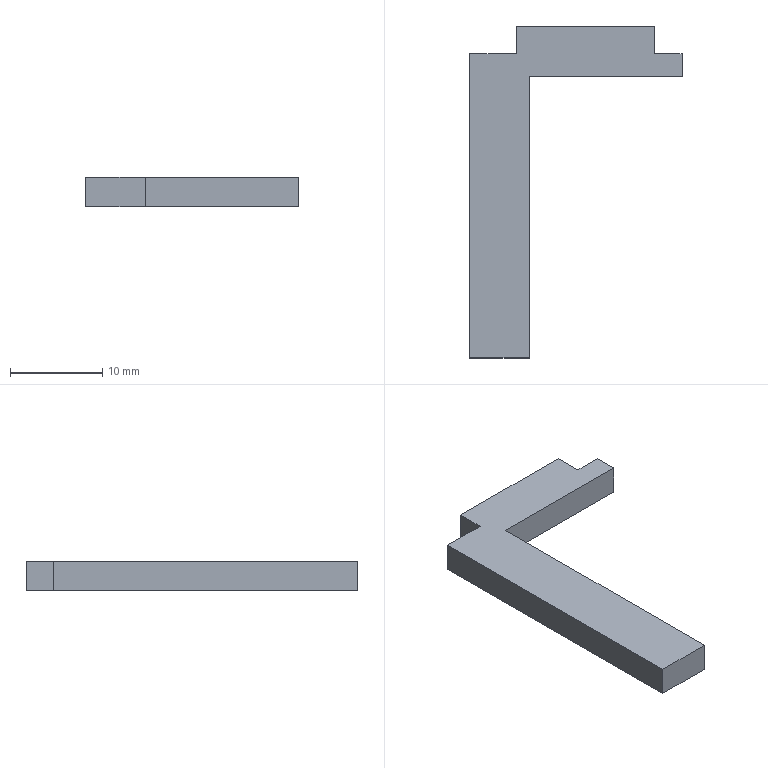Part | SolidWorks | features FlatPattern 1, SMBaseFlange 1, SheetMetal 1 | 1 solid | 12 faces | box 23 x 36 x 3.2 mm | volume 953.226 mm3 | plane 12
STEP:
#1=CARTESIAN_POINT('',(2.154,0.,0.));
#2=VERTEX_POINT('',#1);
#3=CARTESIAN_POINT('',(-0.8457,0.,0.));
#4=VERTEX_POINT('',#3);
#5=CARTESIAN_POINT('',(2.154,0.,0.));
#6=DIRECTION('',(-1.,0.,0.));
#7=VECTOR('',#6,1000.);
#8=LINE('',#5,#7);
#9=EDGE_CURVE('',#2,#4,#8,.T.);
#10=ORIENTED_EDGE('',*,*,#9,.T.);
#11=CARTESIAN_POINT('',(-0.8457,0.,3.2));
#12=VERTEX_POINT('',#11);
#13=CARTESIAN_POINT('',(-0.8457,0.,3.2));
#14=DIRECTION('',(0.,0.,-1.));
#15=VECTOR('',#14,1000.);
#16=LINE('',#13,#15);
#17=EDGE_CURVE('',#12,#4,#16,.T.);
#18=ORIENTED_EDGE('',*,*,#17,.F.);
#19=CARTESIAN_POINT('',(2.154,0.,3.2));
#20=VERTEX_POINT('',#19);
#21=CARTESIAN_POINT('',(2.154,0.,3.2));
#22=DIRECTION('',(-1.,0.,0.));
#23=VECTOR('',#22,1000.);
#24=LINE('',#21,#23);
#25=EDGE_CURVE('',#20,#12,#24,.T.);
#26=ORIENTED_EDGE('',*,*,#25,.F.);
#27=CARTESIAN_POINT('',(2.154,0.,3.2));
#28=DIRECTION('',(0.,0.,-1.));
#29=VECTOR('',#28,1000.);
#30=LINE('',#27,#29);
#31=EDGE_CURVE('',#20,#2,#30,.T.);
#32=ORIENTED_EDGE('',*,*,#31,.T.);
#33=EDGE_LOOP('',(#10,#18,#26,#32));
#34=FACE_OUTER_BOUND('',#33,.T.);
#35=CARTESIAN_POINT('',(2.154,0.,3.2));
#36=DIRECTION('',(0.,-1.,0.));
#37=DIRECTION('',(0.,0.,-1.));
#38=AXIS2_PLACEMENT_3D('',#35,#36,#37);
#39=PLANE('',#38);
#40=ADVANCED_FACE('',(#34),#39,.F.);
#41=CARTESIAN_POINT('',(-0.8457,3.,0.));
#42=VERTEX_POINT('',#41);
#43=CARTESIAN_POINT('',(-0.8457,0.,0.));
#44=DIRECTION('',(0.,1.,0.));
#45=VECTOR('',#44,1000.);
#46=LINE('',#43,#45);
#47=EDGE_CURVE('',#4,#42,#46,.T.);
#48=ORIENTED_EDGE('',*,*,#47,.T.);
#49=CARTESIAN_POINT('',(-0.8457,3.,3.2));
#50=VERTEX_POINT('',#49);
#51=CARTESIAN_POINT('',(-0.8457,3.,3.2));
#52=DIRECTION('',(0.,0.,-1.));
#53=VECTOR('',#52,1000.);
#54=LINE('',#51,#53);
#55=EDGE_CURVE('',#50,#42,#54,.T.);
#56=ORIENTED_EDGE('',*,*,#55,.F.);
#57=CARTESIAN_POINT('',(-0.8457,0.,3.2));
#58=DIRECTION('',(0.,1.,0.));
#59=VECTOR('',#58,1000.);
#60=LINE('',#57,#59);
#61=EDGE_CURVE('',#12,#50,#60,.T.);
#62=ORIENTED_EDGE('',*,*,#61,.F.);
#63=ORIENTED_EDGE('',*,*,#17,.T.);
#64=EDGE_LOOP('',(#48,#56,#62,#63));
#65=FACE_OUTER_BOUND('',#64,.T.);
#66=CARTESIAN_POINT('',(-0.8457,0.,3.2));
#67=DIRECTION('',(-1.,0.,0.));
#68=DIRECTION('',(0.,-1.,0.));
#69=AXIS2_PLACEMENT_3D('',#66,#67,#68);
#70=PLANE('',#69);
#71=ADVANCED_FACE('',(#65),#70,.F.);
#72=CARTESIAN_POINT('',(-15.846,3.,0.));
#73=VERTEX_POINT('',#72);
#74=CARTESIAN_POINT('',(-0.8457,3.,0.));
#75=DIRECTION('',(-1.,0.,0.));
#76=VECTOR('',#75,1000.);
#77=LINE('',#74,#76);
#78=EDGE_CURVE('',#42,#73,#77,.T.);
#79=ORIENTED_EDGE('',*,*,#78,.T.);
#80=CARTESIAN_POINT('',(-15.846,3.,3.2));
#81=VERTEX_POINT('',#80);
#82=CARTESIAN_POINT('',(-15.846,3.,3.2));
#83=DIRECTION('',(0.,0.,-1.));
#84=VECTOR('',#83,1000.);
#85=LINE('',#82,#84);
#86=EDGE_CURVE('',#81,#73,#85,.T.);
#87=ORIENTED_EDGE('',*,*,#86,.F.);
#88=CARTESIAN_POINT('',(-0.8457,3.,3.2));
#89=DIRECTION('',(-1.,0.,0.));
#90=VECTOR('',#89,1000.);
#91=LINE('',#88,#90);
#92=EDGE_CURVE('',#50,#81,#91,.T.);
#93=ORIENTED_EDGE('',*,*,#92,.F.);
#94=ORIENTED_EDGE('',*,*,#55,.T.);
#95=EDGE_LOOP('',(#79,#87,#93,#94));
#96=FACE_OUTER_BOUND('',#95,.T.);
#97=CARTESIAN_POINT('',(-0.8457,3.,3.2));
#98=DIRECTION('',(0.,-1.,0.));
#99=DIRECTION('',(1.,0.,0.));
#100=AXIS2_PLACEMENT_3D('',#97,#98,#99);
#101=PLANE('',#100);
#102=ADVANCED_FACE('',(#96),#101,.F.);
#103=CARTESIAN_POINT('',(-15.846,0.,0.));
#104=VERTEX_POINT('',#103);
#105=CARTESIAN_POINT('',(-15.846,3.,0.));
#106=DIRECTION('',(0.,-1.,0.));
#107=VECTOR('',#106,1000.);
#108=LINE('',#105,#107);
#109=EDGE_CURVE('',#73,#104,#108,.T.);
#110=ORIENTED_EDGE('',*,*,#109,.T.);
#111=CARTESIAN_POINT('',(-15.846,0.,3.2));
#112=VERTEX_POINT('',#111);
#113=CARTESIAN_POINT('',(-15.846,0.,3.2));
#114=DIRECTION('',(0.,0.,-1.));
#115=VECTOR('',#114,1000.);
#116=LINE('',#113,#115);
#117=EDGE_CURVE('',#112,#104,#116,.T.);
#118=ORIENTED_EDGE('',*,*,#117,.F.);
#119=CARTESIAN_POINT('',(-15.846,3.,3.2));
#120=DIRECTION('',(0.,-1.,0.));
#121=VECTOR('',#120,1000.);
#122=LINE('',#119,#121);
#123=EDGE_CURVE('',#81,#112,#122,.T.);
#124=ORIENTED_EDGE('',*,*,#123,.F.);
#125=ORIENTED_EDGE('',*,*,#86,.T.);
#126=EDGE_LOOP('',(#110,#118,#124,#125));
#127=FACE_OUTER_BOUND('',#126,.T.);
#128=CARTESIAN_POINT('',(-15.846,3.,3.2));
#129=DIRECTION('',(1.,0.,0.));
#130=DIRECTION('',(0.,0.,-1.));
#131=AXIS2_PLACEMENT_3D('',#128,#129,#130);
#132=PLANE('',#131);
#133=ADVANCED_FACE('',(#127),#132,.F.);
#134=CARTESIAN_POINT('',(-20.846,0.,0.));
#135=VERTEX_POINT('',#134);
#136=CARTESIAN_POINT('',(-15.846,0.,0.));
#137=DIRECTION('',(-1.,0.,0.));
#138=VECTOR('',#137,1000.);
#139=LINE('',#136,#138);
#140=EDGE_CURVE('',#104,#135,#139,.T.);
#141=ORIENTED_EDGE('',*,*,#140,.T.);
#142=CARTESIAN_POINT('',(-20.846,0.,3.2));
#143=VERTEX_POINT('',#142);
#144=CARTESIAN_POINT('',(-20.846,0.,3.2));
#145=DIRECTION('',(0.,0.,-1.));
#146=VECTOR('',#145,1000.);
#147=LINE('',#144,#146);
#148=EDGE_CURVE('',#143,#135,#147,.T.);
#149=ORIENTED_EDGE('',*,*,#148,.F.);
#150=CARTESIAN_POINT('',(-15.846,0.,3.2));
#151=DIRECTION('',(-1.,0.,0.));
#152=VECTOR('',#151,1000.);
#153=LINE('',#150,#152);
#154=EDGE_CURVE('',#112,#143,#153,.T.);
#155=ORIENTED_EDGE('',*,*,#154,.F.);
#156=ORIENTED_EDGE('',*,*,#117,.T.);
#157=EDGE_LOOP('',(#141,#149,#155,#156));
#158=FACE_OUTER_BOUND('',#157,.T.);
#159=CARTESIAN_POINT('',(-15.846,0.,3.2));
#160=DIRECTION('',(0.,-1.,0.));
#161=DIRECTION('',(1.,0.,0.));
#162=AXIS2_PLACEMENT_3D('',#159,#160,#161);
#163=PLANE('',#162);
#164=ADVANCED_FACE('',(#158),#163,.F.);
#165=CARTESIAN_POINT('',(-20.846,-33.,0.));
#166=VERTEX_POINT('',#165);
#167=CARTESIAN_POINT('',(-20.846,0.,0.));
#168=DIRECTION('',(0.,-1.,0.));
#169=VECTOR('',#168,1000.);
#170=LINE('',#167,#169);
#171=EDGE_CURVE('',#135,#166,#170,.T.);
#172=ORIENTED_EDGE('',*,*,#171,.T.);
#173=CARTESIAN_POINT('',(-20.846,-33.,3.2));
#174=VERTEX_POINT('',#173);
#175=CARTESIAN_POINT('',(-20.846,-33.,3.2));
#176=DIRECTION('',(0.,0.,-1.));
#177=VECTOR('',#176,1000.);
#178=LINE('',#175,#177);
#179=EDGE_CURVE('',#174,#166,#178,.T.);
#180=ORIENTED_EDGE('',*,*,#179,.F.);
#181=CARTESIAN_POINT('',(-20.846,0.,3.2));
#182=DIRECTION('',(0.,-1.,0.));
#183=VECTOR('',#182,1000.);
#184=LINE('',#181,#183);
#185=EDGE_CURVE('',#143,#174,#184,.T.);
#186=ORIENTED_EDGE('',*,*,#185,.F.);
#187=ORIENTED_EDGE('',*,*,#148,.T.);
#188=EDGE_LOOP('',(#172,#180,#186,#187));
#189=FACE_OUTER_BOUND('',#188,.T.);
#190=CARTESIAN_POINT('',(-20.846,0.,3.2));
#191=DIRECTION('',(1.,0.,0.));
#192=DIRECTION('',(0.,1.,0.));
#193=AXIS2_PLACEMENT_3D('',#190,#191,#192);
#194=PLANE('',#193);
#195=ADVANCED_FACE('',(#189),#194,.F.);
#196=CARTESIAN_POINT('',(-14.44,-33.,0.));
#197=VERTEX_POINT('',#196);
#198=CARTESIAN_POINT('',(-20.846,-33.,0.));
#199=DIRECTION('',(1.,0.,0.));
#200=VECTOR('',#199,1000.);
#201=LINE('',#198,#200);
#202=EDGE_CURVE('',#166,#197,#201,.T.);
#203=ORIENTED_EDGE('',*,*,#202,.T.);
#204=CARTESIAN_POINT('',(-14.44,-33.,3.2));
#205=VERTEX_POINT('',#204);
#206=CARTESIAN_POINT('',(-14.44,-33.,3.2));
#207=DIRECTION('',(0.,0.,-1.));
#208=VECTOR('',#207,1000.);
#209=LINE('',#206,#208);
#210=EDGE_CURVE('',#205,#197,#209,.T.);
#211=ORIENTED_EDGE('',*,*,#210,.F.);
#212=CARTESIAN_POINT('',(-20.846,-33.,3.2));
#213=DIRECTION('',(1.,0.,0.));
#214=VECTOR('',#213,1000.);
#215=LINE('',#212,#214);
#216=EDGE_CURVE('',#174,#205,#215,.T.);
#217=ORIENTED_EDGE('',*,*,#216,.F.);
#218=ORIENTED_EDGE('',*,*,#179,.T.);
#219=EDGE_LOOP('',(#203,#211,#217,#218));
#220=FACE_OUTER_BOUND('',#219,.T.);
#221=CARTESIAN_POINT('',(-20.846,-33.,3.2));
#222=DIRECTION('',(0.,1.,0.));
#223=DIRECTION('',(0.,0.,1.));
#224=AXIS2_PLACEMENT_3D('',#221,#222,#223);
#225=PLANE('',#224);
#226=ADVANCED_FACE('',(#220),#225,.F.);
#227=CARTESIAN_POINT('',(-14.44,-2.5,0.));
#228=VERTEX_POINT('',#227);
#229=CARTESIAN_POINT('',(-14.44,-33.,0.));
#230=DIRECTION('',(0.,1.,0.));
#231=VECTOR('',#230,1000.);
#232=LINE('',#229,#231);
#233=EDGE_CURVE('',#197,#228,#232,.T.);
#234=ORIENTED_EDGE('',*,*,#233,.T.);
#235=CARTESIAN_POINT('',(-14.44,-2.5,3.2));
#236=VERTEX_POINT('',#235);
#237=CARTESIAN_POINT('',(-14.44,-2.5,3.2));
#238=DIRECTION('',(0.,0.,-1.));
#239=VECTOR('',#238,1000.);
#240=LINE('',#237,#239);
#241=EDGE_CURVE('',#236,#228,#240,.T.);
#242=ORIENTED_EDGE('',*,*,#241,.F.);
#243=CARTESIAN_POINT('',(-14.44,-33.,3.2));
#244=DIRECTION('',(0.,1.,0.));
#245=VECTOR('',#244,1000.);
#246=LINE('',#243,#245);
#247=EDGE_CURVE('',#205,#236,#246,.T.);
#248=ORIENTED_EDGE('',*,*,#247,.F.);
#249=ORIENTED_EDGE('',*,*,#210,.T.);
#250=EDGE_LOOP('',(#234,#242,#248,#249));
#251=FACE_OUTER_BOUND('',#250,.T.);
#252=CARTESIAN_POINT('',(-14.44,-33.,3.2));
#253=DIRECTION('',(-1.,0.,0.));
#254=DIRECTION('',(0.,0.,1.));
#255=AXIS2_PLACEMENT_3D('',#252,#253,#254);
#256=PLANE('',#255);
#257=ADVANCED_FACE('',(#251),#256,.F.);
#258=CARTESIAN_POINT('',(2.154,-2.5,0.));
#259=VERTEX_POINT('',#258);
#260=CARTESIAN_POINT('',(2.154,-2.5,0.));
#261=DIRECTION('',(1.,0.,0.));
#262=VECTOR('',#261,1000.);
#263=LINE('',#260,#262);
#264=EDGE_CURVE('',#228,#259,#263,.T.);
#265=ORIENTED_EDGE('',*,*,#264,.T.);
#266=CARTESIAN_POINT('',(2.154,-2.5,3.2));
#267=VERTEX_POINT('',#266);
#268=CARTESIAN_POINT('',(2.154,-2.5,3.2));
#269=DIRECTION('',(0.,0.,-1.));
#270=VECTOR('',#269,1000.);
#271=LINE('',#268,#270);
#272=EDGE_CURVE('',#267,#259,#271,.T.);
#273=ORIENTED_EDGE('',*,*,#272,.F.);
#274=CARTESIAN_POINT('',(2.154,-2.5,3.2));
#275=DIRECTION('',(1.,0.,0.));
#276=VECTOR('',#275,1000.);
#277=LINE('',#274,#276);
#278=EDGE_CURVE('',#236,#267,#277,.T.);
#279=ORIENTED_EDGE('',*,*,#278,.F.);
#280=ORIENTED_EDGE('',*,*,#241,.T.);
#281=EDGE_LOOP('',(#265,#273,#279,#280));
#282=FACE_OUTER_BOUND('',#281,.T.);
#283=CARTESIAN_POINT('',(2.154,-2.5,3.2));
#284=DIRECTION('',(0.,1.,0.));
#285=DIRECTION('',(-1.,0.,0.));
#286=AXIS2_PLACEMENT_3D('',#283,#284,#285);
#287=PLANE('',#286);
#288=ADVANCED_FACE('',(#282),#287,.F.);
#289=CARTESIAN_POINT('',(2.154,-2.5,0.));
#290=DIRECTION('',(0.,1.,0.));
#291=VECTOR('',#290,1000.);
#292=LINE('',#289,#291);
#293=EDGE_CURVE('',#259,#2,#292,.T.);
#294=ORIENTED_EDGE('',*,*,#293,.T.);
#295=ORIENTED_EDGE('',*,*,#31,.F.);
#296=CARTESIAN_POINT('',(2.154,-2.5,3.2));
#297=DIRECTION('',(0.,1.,0.));
#298=VECTOR('',#297,1000.);
#299=LINE('',#296,#298);
#300=EDGE_CURVE('',#267,#20,#299,.T.);
#301=ORIENTED_EDGE('',*,*,#300,.F.);
#302=ORIENTED_EDGE('',*,*,#272,.T.);
#303=EDGE_LOOP('',(#294,#295,#301,#302));
#304=FACE_OUTER_BOUND('',#303,.T.);
#305=CARTESIAN_POINT('',(2.154,-2.5,3.2));
#306=DIRECTION('',(-1.,0.,0.));
#307=DIRECTION('',(0.,-1.,0.));
#308=AXIS2_PLACEMENT_3D('',#305,#306,#307);
#309=PLANE('',#308);
#310=ADVANCED_FACE('',(#304),#309,.F.);
#311=ORIENTED_EDGE('',*,*,#25,.T.);
#312=ORIENTED_EDGE('',*,*,#61,.T.);
#313=ORIENTED_EDGE('',*,*,#92,.T.);
#314=ORIENTED_EDGE('',*,*,#123,.T.);
#315=ORIENTED_EDGE('',*,*,#154,.T.);
#316=ORIENTED_EDGE('',*,*,#185,.T.);
#317=ORIENTED_EDGE('',*,*,#216,.T.);
#318=ORIENTED_EDGE('',*,*,#247,.T.);
#319=ORIENTED_EDGE('',*,*,#278,.T.);
#320=ORIENTED_EDGE('',*,*,#300,.T.);
#321=EDGE_LOOP('',(#311,#312,#313,#314,#315,#316,#317,#318,#319,#320));
#322=FACE_OUTER_BOUND('',#321,.T.);
#323=CARTESIAN_POINT('',(0.,0.,3.2));
#324=DIRECTION('',(0.,0.,-1.));
#325=DIRECTION('',(-1.,0.,0.));
#326=AXIS2_PLACEMENT_3D('',#323,#324,#325);
#327=PLANE('',#326);
#328=ADVANCED_FACE('',(#322),#327,.F.);
#329=ORIENTED_EDGE('',*,*,#9,.F.);
#330=ORIENTED_EDGE('',*,*,#293,.F.);
#331=ORIENTED_EDGE('',*,*,#264,.F.);
#332=ORIENTED_EDGE('',*,*,#233,.F.);
#333=ORIENTED_EDGE('',*,*,#202,.F.);
#334=ORIENTED_EDGE('',*,*,#171,.F.);
#335=ORIENTED_EDGE('',*,*,#140,.F.);
#336=ORIENTED_EDGE('',*,*,#109,.F.);
#337=ORIENTED_EDGE('',*,*,#78,.F.);
#338=ORIENTED_EDGE('',*,*,#47,.F.);
#339=EDGE_LOOP('',(#329,#330,#331,#332,#333,#334,#335,#336,#337,#338));
#340=FACE_OUTER_BOUND('',#339,.T.);
#341=CARTESIAN_POINT('',(0.,0.,0.));
#342=DIRECTION('',(0.,0.,-1.));
#343=DIRECTION('',(-1.,0.,0.));
#344=AXIS2_PLACEMENT_3D('',#341,#342,#343);
#345=PLANE('',#344);
#346=ADVANCED_FACE('',(#340),#345,.T.);
#347=CLOSED_SHELL('',(#40,#71,#102,#133,#164,#195,#226,#257,#288,#310,#328,#346));
#348=MANIFOLD_SOLID_BREP('',#347);
#349=CARTESIAN_POINT('',(0.,0.,0.));
#350=DIRECTION('',(0.,0.,1.));
#351=DIRECTION('',(1.,0.,0.));
#352=AXIS2_PLACEMENT_3D('',#349,#350,#351);
#353=(LENGTH_UNIT()NAMED_UNIT(*)SI_UNIT(.MILLI.,.METRE.));
#354=UNCERTAINTY_MEASURE_WITH_UNIT(LENGTH_MEASURE(0.00001),#353,'','');
#355=(NAMED_UNIT(*)PLANE_ANGLE_UNIT()SI_UNIT($,.RADIAN.));
#356=(NAMED_UNIT(*)SI_UNIT($,.STERADIAN.)SOLID_ANGLE_UNIT());
#357=(GEOMETRIC_REPRESENTATION_CONTEXT(3)GLOBAL_UNCERTAINTY_ASSIGNED_CONTEXT((#354))GLOBAL_UNIT_ASSIGNED_CONTEXT((#353,#355,#356))REPRESENTATION_CONTEXT('',''));
#358=ADVANCED_BREP_SHAPE_REPRESENTATION('',(#348,#352),#357);